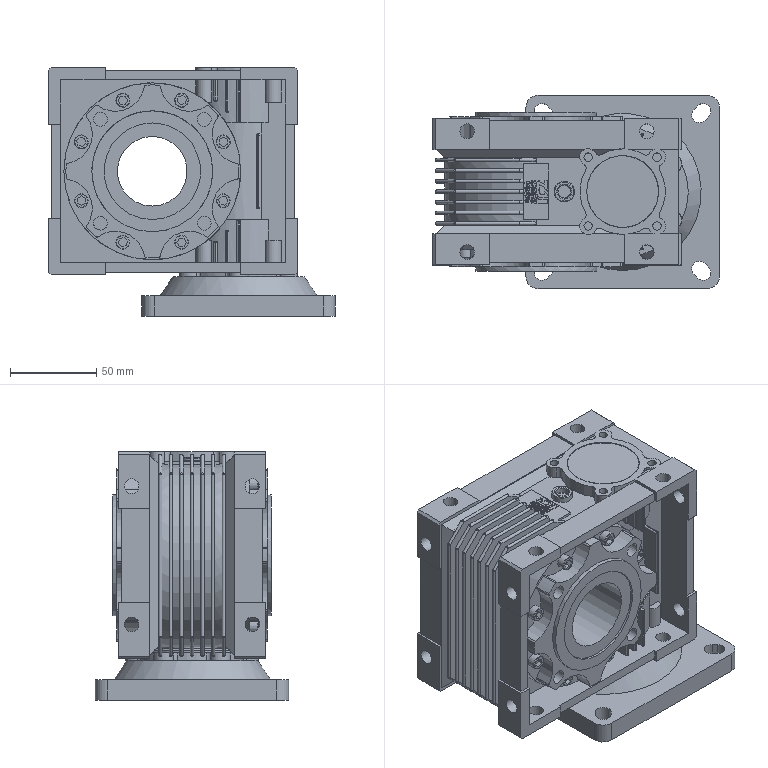Part | STEP file | 冲床-300配套压波_id1122_x_t | 1 solid | 1325 faces | box 166 x 112 x 144 mm | volume 998594 mm3 | plane 719 | cylinder 449 | sphere 73 | other 61 | torus 14 | cone 9 | commonest cylinder face diameters 1.96 x72 2 x72 1.5 x66 4.9 x20 12 x18 8 x16